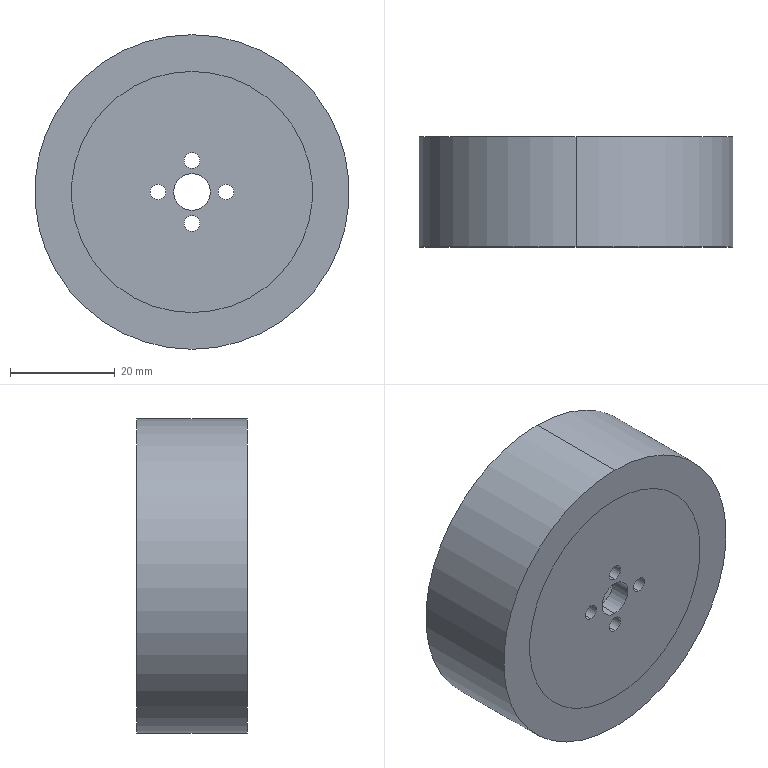Part | SolidWorks | features ICE 2, Extrusion 1 | 2 solids | 23 faces | box 60 x 21 x 60 mm | volume 35557 mm3 | cylinder 18 | plane 5 | commonest cylinder face diameters 3 x8 46 x4 7 x2 42 x2 60 x2
STEP:
#1=CARTESIAN_POINT('',(0.,21.,-21.));
#2=VERTEX_POINT('',#1);
#3=CARTESIAN_POINT('',(0.,21.,21.));
#4=VERTEX_POINT('',#3);
#5=CARTESIAN_POINT('',(0.,21.,0.));
#6=DIRECTION('',(0.,1.,0.));
#7=DIRECTION('',(0.,0.,1.));
#8=AXIS2_PLACEMENT_3D('',#5,#6,#7);
#9=CIRCLE('',#8,21.);
#10=EDGE_CURVE('',#2,#4,#9,.T.);
#11=ORIENTED_EDGE('',*,*,#10,.T.);
#12=CARTESIAN_POINT('',(0.,4.,21.));
#13=VERTEX_POINT('',#12);
#14=CARTESIAN_POINT('',(0.,21.,21.));
#15=DIRECTION('',(0.,-1.,0.));
#16=VECTOR('',#15,1000.);
#17=LINE('',#14,#16);
#18=EDGE_CURVE('',#4,#13,#17,.T.);
#19=ORIENTED_EDGE('',*,*,#18,.T.);
#20=CARTESIAN_POINT('',(0.,4.,-21.));
#21=VERTEX_POINT('',#20);
#22=CARTESIAN_POINT('',(0.,4.,0.));
#23=DIRECTION('',(0.,-1.,0.));
#24=DIRECTION('',(0.,0.,1.));
#25=AXIS2_PLACEMENT_3D('',#22,#23,#24);
#26=CIRCLE('',#25,21.);
#27=EDGE_CURVE('',#13,#21,#26,.T.);
#28=ORIENTED_EDGE('',*,*,#27,.T.);
#29=CARTESIAN_POINT('',(0.,21.,-21.));
#30=DIRECTION('',(0.,-1.,0.));
#31=VECTOR('',#30,1000.);
#32=LINE('',#29,#31);
#33=EDGE_CURVE('',#2,#21,#32,.T.);
#34=ORIENTED_EDGE('',*,*,#33,.F.);
#35=EDGE_LOOP('',(#11,#19,#28,#34));
#36=FACE_OUTER_BOUND('',#35,.T.);
#37=CARTESIAN_POINT('',(0.,21.,0.));
#38=DIRECTION('',(0.,-1.,0.));
#39=DIRECTION('',(0.,0.,-1.));
#40=AXIS2_PLACEMENT_3D('',#37,#38,#39);
#41=CYLINDRICAL_SURFACE('',#40,21.);
#42=ADVANCED_FACE('',(#36),#41,.F.);
#43=CARTESIAN_POINT('',(0.,4.,-3.5));
#44=VERTEX_POINT('',#43);
#45=CARTESIAN_POINT('',(0.,4.,3.5));
#46=VERTEX_POINT('',#45);
#47=CARTESIAN_POINT('',(0.,4.,0.));
#48=DIRECTION('',(0.,1.,0.));
#49=DIRECTION('',(0.,0.,1.));
#50=AXIS2_PLACEMENT_3D('',#47,#48,#49);
#51=CIRCLE('',#50,3.5);
#52=EDGE_CURVE('',#44,#46,#51,.T.);
#53=ORIENTED_EDGE('',*,*,#52,.T.);
#54=CARTESIAN_POINT('',(0.,0.,3.5));
#55=VERTEX_POINT('',#54);
#56=CARTESIAN_POINT('',(0.,4.,3.5));
#57=DIRECTION('',(0.,-1.,0.));
#58=VECTOR('',#57,1000.);
#59=LINE('',#56,#58);
#60=EDGE_CURVE('',#46,#55,#59,.T.);
#61=ORIENTED_EDGE('',*,*,#60,.T.);
#62=CARTESIAN_POINT('',(0.,0.,-3.5));
#63=VERTEX_POINT('',#62);
#64=CARTESIAN_POINT('',(0.,0.,0.));
#65=DIRECTION('',(0.,1.,0.));
#66=DIRECTION('',(0.,0.,1.));
#67=AXIS2_PLACEMENT_3D('',#64,#65,#66);
#68=CIRCLE('',#67,3.5);
#69=EDGE_CURVE('',#63,#55,#68,.T.);
#70=ORIENTED_EDGE('',*,*,#69,.F.);
#71=CARTESIAN_POINT('',(0.,4.,-3.5));
#72=DIRECTION('',(0.,-1.,0.));
#73=VECTOR('',#72,1000.);
#74=LINE('',#71,#73);
#75=EDGE_CURVE('',#44,#63,#74,.T.);
#76=ORIENTED_EDGE('',*,*,#75,.F.);
#77=EDGE_LOOP('',(#53,#61,#70,#76));
#78=FACE_OUTER_BOUND('',#77,.T.);
#79=CARTESIAN_POINT('',(0.,4.,0.));
#80=DIRECTION('',(0.,-1.,0.));
#81=DIRECTION('',(0.,0.,-1.));
#82=AXIS2_PLACEMENT_3D('',#79,#80,#81);
#83=CYLINDRICAL_SURFACE('',#82,3.5);
#84=ADVANCED_FACE('',(#78),#83,.F.);
#85=CARTESIAN_POINT('',(0.,4.,-7.5));
#86=VERTEX_POINT('',#85);
#87=CARTESIAN_POINT('',(0.,4.,-4.5));
#88=VERTEX_POINT('',#87);
#89=CARTESIAN_POINT('',(0.,4.,-6.));
#90=DIRECTION('',(0.,1.,0.));
#91=DIRECTION('',(0.,0.,1.));
#92=AXIS2_PLACEMENT_3D('',#89,#90,#91);
#93=CIRCLE('',#92,1.5);
#94=EDGE_CURVE('',#86,#88,#93,.T.);
#95=ORIENTED_EDGE('',*,*,#94,.T.);
#96=CARTESIAN_POINT('',(0.,0.,-4.5));
#97=VERTEX_POINT('',#96);
#98=CARTESIAN_POINT('',(0.,4.,-4.5));
#99=DIRECTION('',(0.,-1.,0.));
#100=VECTOR('',#99,1000.);
#101=LINE('',#98,#100);
#102=EDGE_CURVE('',#88,#97,#101,.T.);
#103=ORIENTED_EDGE('',*,*,#102,.T.);
#104=CARTESIAN_POINT('',(0.,0.,-7.5));
#105=VERTEX_POINT('',#104);
#106=CARTESIAN_POINT('',(0.,0.,-6.));
#107=DIRECTION('',(0.,1.,0.));
#108=DIRECTION('',(0.,0.,1.));
#109=AXIS2_PLACEMENT_3D('',#106,#107,#108);
#110=CIRCLE('',#109,1.5);
#111=EDGE_CURVE('',#105,#97,#110,.T.);
#112=ORIENTED_EDGE('',*,*,#111,.F.);
#113=CARTESIAN_POINT('',(0.,4.,-7.5));
#114=DIRECTION('',(0.,-1.,0.));
#115=VECTOR('',#114,1000.);
#116=LINE('',#113,#115);
#117=EDGE_CURVE('',#86,#105,#116,.T.);
#118=ORIENTED_EDGE('',*,*,#117,.F.);
#119=EDGE_LOOP('',(#95,#103,#112,#118));
#120=FACE_OUTER_BOUND('',#119,.T.);
#121=CARTESIAN_POINT('',(0.,4.,-6.));
#122=DIRECTION('',(0.,-1.,0.));
#123=DIRECTION('',(0.,0.,-1.));
#124=AXIS2_PLACEMENT_3D('',#121,#122,#123);
#125=CYLINDRICAL_SURFACE('',#124,1.5);
#126=ADVANCED_FACE('',(#120),#125,.F.);
#127=CARTESIAN_POINT('',(0.,4.,4.5));
#128=VERTEX_POINT('',#127);
#129=CARTESIAN_POINT('',(0.,4.,7.5));
#130=VERTEX_POINT('',#129);
#131=CARTESIAN_POINT('',(0.,4.,6.));
#132=DIRECTION('',(0.,1.,0.));
#133=DIRECTION('',(0.,0.,1.));
#134=AXIS2_PLACEMENT_3D('',#131,#132,#133);
#135=CIRCLE('',#134,1.5);
#136=EDGE_CURVE('',#128,#130,#135,.T.);
#137=ORIENTED_EDGE('',*,*,#136,.T.);
#138=CARTESIAN_POINT('',(0.,0.,7.5));
#139=VERTEX_POINT('',#138);
#140=CARTESIAN_POINT('',(0.,4.,7.5));
#141=DIRECTION('',(0.,-1.,0.));
#142=VECTOR('',#141,1000.);
#143=LINE('',#140,#142);
#144=EDGE_CURVE('',#130,#139,#143,.T.);
#145=ORIENTED_EDGE('',*,*,#144,.T.);
#146=CARTESIAN_POINT('',(0.,0.,4.5));
#147=VERTEX_POINT('',#146);
#148=CARTESIAN_POINT('',(0.,0.,6.));
#149=DIRECTION('',(0.,1.,0.));
#150=DIRECTION('',(0.,0.,1.));
#151=AXIS2_PLACEMENT_3D('',#148,#149,#150);
#152=CIRCLE('',#151,1.5);
#153=EDGE_CURVE('',#147,#139,#152,.T.);
#154=ORIENTED_EDGE('',*,*,#153,.F.);
#155=CARTESIAN_POINT('',(0.,4.,4.5));
#156=DIRECTION('',(0.,-1.,0.));
#157=VECTOR('',#156,1000.);
#158=LINE('',#155,#157);
#159=EDGE_CURVE('',#128,#147,#158,.T.);
#160=ORIENTED_EDGE('',*,*,#159,.F.);
#161=EDGE_LOOP('',(#137,#145,#154,#160));
#162=FACE_OUTER_BOUND('',#161,.T.);
#163=CARTESIAN_POINT('',(0.,4.,6.));
#164=DIRECTION('',(0.,-1.,0.));
#165=DIRECTION('',(0.,0.,-1.));
#166=AXIS2_PLACEMENT_3D('',#163,#164,#165);
#167=CYLINDRICAL_SURFACE('',#166,1.5);
#168=ADVANCED_FACE('',(#162),#167,.F.);
#169=CARTESIAN_POINT('',(-6.5,4.,-1.5));
#170=VERTEX_POINT('',#169);
#171=CARTESIAN_POINT('',(-6.5,4.,1.5));
#172=VERTEX_POINT('',#171);
#173=CARTESIAN_POINT('',(-6.5,4.,0.));
#174=DIRECTION('',(0.,1.,0.));
#175=DIRECTION('',(0.,0.,1.));
#176=AXIS2_PLACEMENT_3D('',#173,#174,#175);
#177=CIRCLE('',#176,1.5);
#178=EDGE_CURVE('',#170,#172,#177,.T.);
#179=ORIENTED_EDGE('',*,*,#178,.T.);
#180=CARTESIAN_POINT('',(-6.5,0.,1.5));
#181=VERTEX_POINT('',#180);
#182=CARTESIAN_POINT('',(-6.5,4.,1.5));
#183=DIRECTION('',(0.,-1.,0.));
#184=VECTOR('',#183,1000.);
#185=LINE('',#182,#184);
#186=EDGE_CURVE('',#172,#181,#185,.T.);
#187=ORIENTED_EDGE('',*,*,#186,.T.);
#188=CARTESIAN_POINT('',(-6.5,0.,-1.5));
#189=VERTEX_POINT('',#188);
#190=CARTESIAN_POINT('',(-6.5,0.,0.));
#191=DIRECTION('',(0.,1.,0.));
#192=DIRECTION('',(0.,0.,1.));
#193=AXIS2_PLACEMENT_3D('',#190,#191,#192);
#194=CIRCLE('',#193,1.5);
#195=EDGE_CURVE('',#189,#181,#194,.T.);
#196=ORIENTED_EDGE('',*,*,#195,.F.);
#197=CARTESIAN_POINT('',(-6.5,4.,-1.5));
#198=DIRECTION('',(0.,-1.,0.));
#199=VECTOR('',#198,1000.);
#200=LINE('',#197,#199);
#201=EDGE_CURVE('',#170,#189,#200,.T.);
#202=ORIENTED_EDGE('',*,*,#201,.F.);
#203=EDGE_LOOP('',(#179,#187,#196,#202));
#204=FACE_OUTER_BOUND('',#203,.T.);
#205=CARTESIAN_POINT('',(-6.5,4.,0.));
#206=DIRECTION('',(0.,-1.,0.));
#207=DIRECTION('',(0.,0.,-1.));
#208=AXIS2_PLACEMENT_3D('',#205,#206,#207);
#209=CYLINDRICAL_SURFACE('',#208,1.5);
#210=ADVANCED_FACE('',(#204),#209,.F.);
#211=CARTESIAN_POINT('',(6.5,4.,-1.5));
#212=VERTEX_POINT('',#211);
#213=CARTESIAN_POINT('',(6.5,4.,1.5));
#214=VERTEX_POINT('',#213);
#215=CARTESIAN_POINT('',(6.5,4.,0.));
#216=DIRECTION('',(0.,1.,0.));
#217=DIRECTION('',(0.,0.,1.));
#218=AXIS2_PLACEMENT_3D('',#215,#216,#217);
#219=CIRCLE('',#218,1.5);
#220=EDGE_CURVE('',#212,#214,#219,.T.);
#221=ORIENTED_EDGE('',*,*,#220,.T.);
#222=CARTESIAN_POINT('',(6.5,0.,1.5));
#223=VERTEX_POINT('',#222);
#224=CARTESIAN_POINT('',(6.5,4.,1.5));
#225=DIRECTION('',(0.,-1.,0.));
#226=VECTOR('',#225,1000.);
#227=LINE('',#224,#226);
#228=EDGE_CURVE('',#214,#223,#227,.T.);
#229=ORIENTED_EDGE('',*,*,#228,.T.);
#230=CARTESIAN_POINT('',(6.5,0.,-1.5));
#231=VERTEX_POINT('',#230);
#232=CARTESIAN_POINT('',(6.5,0.,0.));
#233=DIRECTION('',(0.,1.,0.));
#234=DIRECTION('',(0.,0.,1.));
#235=AXIS2_PLACEMENT_3D('',#232,#233,#234);
#236=CIRCLE('',#235,1.5);
#237=EDGE_CURVE('',#231,#223,#236,.T.);
#238=ORIENTED_EDGE('',*,*,#237,.F.);
#239=CARTESIAN_POINT('',(6.5,4.,-1.5));
#240=DIRECTION('',(0.,-1.,0.));
#241=VECTOR('',#240,1000.);
#242=LINE('',#239,#241);
#243=EDGE_CURVE('',#212,#231,#242,.T.);
#244=ORIENTED_EDGE('',*,*,#243,.F.);
#245=EDGE_LOOP('',(#221,#229,#238,#244));
#246=FACE_OUTER_BOUND('',#245,.T.);
#247=CARTESIAN_POINT('',(6.5,4.,0.));
#248=DIRECTION('',(0.,-1.,0.));
#249=DIRECTION('',(0.,0.,-1.));
#250=AXIS2_PLACEMENT_3D('',#247,#248,#249);
#251=CYLINDRICAL_SURFACE('',#250,1.5);
#252=ADVANCED_FACE('',(#246),#251,.F.);
#253=CARTESIAN_POINT('',(0.,21.,23.));
#254=VERTEX_POINT('',#253);
#255=CARTESIAN_POINT('',(0.,21.,-23.));
#256=VERTEX_POINT('',#255);
#257=CARTESIAN_POINT('',(0.,21.,0.));
#258=DIRECTION('',(0.,1.,0.));
#259=DIRECTION('',(0.,0.,1.));
#260=AXIS2_PLACEMENT_3D('',#257,#258,#259);
#261=CIRCLE('',#260,23.);
#262=EDGE_CURVE('',#254,#256,#261,.T.);
#263=ORIENTED_EDGE('',*,*,#262,.F.);
#264=CARTESIAN_POINT('',(0.,0.,23.));
#265=VERTEX_POINT('',#264);
#266=CARTESIAN_POINT('',(0.,4.,23.));
#267=DIRECTION('',(0.,-1.,0.));
#268=VECTOR('',#267,1000.);
#269=LINE('',#266,#268);
#270=EDGE_CURVE('',#254,#265,#269,.T.);
#271=ORIENTED_EDGE('',*,*,#270,.T.);
#272=CARTESIAN_POINT('',(0.,0.,-23.));
#273=VERTEX_POINT('',#272);
#274=CARTESIAN_POINT('',(0.,0.,0.));
#275=DIRECTION('',(0.,1.,0.));
#276=DIRECTION('',(0.,0.,1.));
#277=AXIS2_PLACEMENT_3D('',#274,#275,#276);
#278=CIRCLE('',#277,23.);
#279=EDGE_CURVE('',#265,#273,#278,.T.);
#280=ORIENTED_EDGE('',*,*,#279,.T.);
#281=CARTESIAN_POINT('',(0.,4.,-23.));
#282=DIRECTION('',(0.,-1.,0.));
#283=VECTOR('',#282,1000.);
#284=LINE('',#281,#283);
#285=EDGE_CURVE('',#256,#273,#284,.T.);
#286=ORIENTED_EDGE('',*,*,#285,.F.);
#287=EDGE_LOOP('',(#263,#271,#280,#286));
#288=FACE_OUTER_BOUND('',#287,.T.);
#289=CARTESIAN_POINT('',(0.,4.,0.));
#290=DIRECTION('',(0.,-1.,0.));
#291=DIRECTION('',(0.,0.,-1.));
#292=AXIS2_PLACEMENT_3D('',#289,#290,#291);
#293=CYLINDRICAL_SURFACE('',#292,23.);
#294=ADVANCED_FACE('',(#288),#293,.T.);
#295=ORIENTED_EDGE('',*,*,#52,.F.);
#296=CARTESIAN_POINT('',(0.,4.,0.));
#297=DIRECTION('',(0.,1.,0.));
#298=DIRECTION('',(0.,0.,1.));
#299=AXIS2_PLACEMENT_3D('',#296,#297,#298);
#300=CIRCLE('',#299,3.5);
#301=EDGE_CURVE('',#46,#44,#300,.T.);
#302=ORIENTED_EDGE('',*,*,#301,.F.);
#303=EDGE_LOOP('',(#295,#302));
#304=FACE_BOUND('',#303,.T.);
#305=ORIENTED_EDGE('',*,*,#136,.F.);
#306=CARTESIAN_POINT('',(0.,4.,6.));
#307=DIRECTION('',(0.,1.,0.));
#308=DIRECTION('',(0.,0.,1.));
#309=AXIS2_PLACEMENT_3D('',#306,#307,#308);
#310=CIRCLE('',#309,1.5);
#311=EDGE_CURVE('',#130,#128,#310,.T.);
#312=ORIENTED_EDGE('',*,*,#311,.F.);
#313=EDGE_LOOP('',(#305,#312));
#314=FACE_BOUND('',#313,.T.);
#315=ORIENTED_EDGE('',*,*,#220,.F.);
#316=CARTESIAN_POINT('',(6.5,4.,0.));
#317=DIRECTION('',(0.,1.,0.));
#318=DIRECTION('',(0.,0.,1.));
#319=AXIS2_PLACEMENT_3D('',#316,#317,#318);
#320=CIRCLE('',#319,1.5);
#321=EDGE_CURVE('',#214,#212,#320,.T.);
#322=ORIENTED_EDGE('',*,*,#321,.F.);
#323=EDGE_LOOP('',(#315,#322));
#324=FACE_BOUND('',#323,.T.);
#325=ORIENTED_EDGE('',*,*,#178,.F.);
#326=CARTESIAN_POINT('',(-6.5,4.,0.));
#327=DIRECTION('',(0.,1.,0.));
#328=DIRECTION('',(0.,0.,1.));
#329=AXIS2_PLACEMENT_3D('',#326,#327,#328);
#330=CIRCLE('',#329,1.5);
#331=EDGE_CURVE('',#172,#170,#330,.T.);
#332=ORIENTED_EDGE('',*,*,#331,.F.);
#333=EDGE_LOOP('',(#325,#332));
#334=FACE_BOUND('',#333,.T.);
#335=ORIENTED_EDGE('',*,*,#94,.F.);
#336=CARTESIAN_POINT('',(0.,4.,-6.));
#337=DIRECTION('',(0.,1.,0.));
#338=DIRECTION('',(0.,0.,1.));
#339=AXIS2_PLACEMENT_3D('',#336,#337,#338);
#340=CIRCLE('',#339,1.5);
#341=EDGE_CURVE('',#88,#86,#340,.T.);
#342=ORIENTED_EDGE('',*,*,#341,.F.);
#343=EDGE_LOOP('',(#335,#342));
#344=FACE_BOUND('',#343,.T.);
#345=CARTESIAN_POINT('',(0.,4.,0.));
#346=DIRECTION('',(0.,-1.,0.));
#347=DIRECTION('',(0.,0.,1.));
#348=AXIS2_PLACEMENT_3D('',#345,#346,#347);
#349=CIRCLE('',#348,21.);
#350=EDGE_CURVE('',#21,#13,#349,.T.);
#351=ORIENTED_EDGE('',*,*,#350,.F.);
#352=ORIENTED_EDGE('',*,*,#27,.F.);
#353=EDGE_LOOP('',(#351,#352));
#354=FACE_OUTER_BOUND('',#353,.T.);
#355=CARTESIAN_POINT('',(0.,4.,0.));
#356=DIRECTION('',(0.,1.,0.));
#357=DIRECTION('',(0.,0.,1.));
#358=AXIS2_PLACEMENT_3D('',#355,#356,#357);
#359=PLANE('',#358);
#360=ADVANCED_FACE('',(#304,#314,#324,#334,#344,#354),#359,.T.);
#361=CARTESIAN_POINT('',(0.,0.,0.));
#362=DIRECTION('',(0.,1.,0.));
#363=DIRECTION('',(0.,0.,1.));
#364=AXIS2_PLACEMENT_3D('',#361,#362,#363);
#365=CIRCLE('',#364,23.);
#366=EDGE_CURVE('',#273,#265,#365,.T.);
#367=ORIENTED_EDGE('',*,*,#366,.F.);
#368=ORIENTED_EDGE('',*,*,#279,.F.);
#369=EDGE_LOOP('',(#367,#368));
#370=FACE_OUTER_BOUND('',#369,.T.);
#371=ORIENTED_EDGE('',*,*,#237,.T.);
#372=CARTESIAN_POINT('',(6.5,0.,0.));
#373=DIRECTION('',(0.,1.,0.));
#374=DIRECTION('',(0.,0.,1.));
#375=AXIS2_PLACEMENT_3D('',#372,#373,#374);
#376=CIRCLE('',#375,1.5);
#377=EDGE_CURVE('',#223,#231,#376,.T.);
#378=ORIENTED_EDGE('',*,*,#377,.T.);
#379=EDGE_LOOP('',(#371,#378));
#380=FACE_BOUND('',#379,.T.);
#381=ORIENTED_EDGE('',*,*,#195,.T.);
#382=CARTESIAN_POINT('',(-6.5,0.,0.));
#383=DIRECTION('',(0.,1.,0.));
#384=DIRECTION('',(0.,0.,1.));
#385=AXIS2_PLACEMENT_3D('',#382,#383,#384);
#386=CIRCLE('',#385,1.5);
#387=EDGE_CURVE('',#181,#189,#386,.T.);
#388=ORIENTED_EDGE('',*,*,#387,.T.);
#389=EDGE_LOOP('',(#381,#388));
#390=FACE_BOUND('',#389,.T.);
#391=ORIENTED_EDGE('',*,*,#153,.T.);
#392=CARTESIAN_POINT('',(0.,0.,6.));
#393=DIRECTION('',(0.,1.,0.));
#394=DIRECTION('',(0.,0.,1.));
#395=AXIS2_PLACEMENT_3D('',#392,#393,#394);
#396=CIRCLE('',#395,1.5);
#397=EDGE_CURVE('',#139,#147,#396,.T.);
#398=ORIENTED_EDGE('',*,*,#397,.T.);
#399=EDGE_LOOP('',(#391,#398));
#400=FACE_BOUND('',#399,.T.);
#401=ORIENTED_EDGE('',*,*,#111,.T.);
#402=CARTESIAN_POINT('',(0.,0.,-6.));
#403=DIRECTION('',(0.,1.,0.));
#404=DIRECTION('',(0.,0.,1.));
#405=AXIS2_PLACEMENT_3D('',#402,#403,#404);
#406=CIRCLE('',#405,1.5);
#407=EDGE_CURVE('',#97,#105,#406,.T.);
#408=ORIENTED_EDGE('',*,*,#407,.T.);
#409=EDGE_LOOP('',(#401,#408));
#410=FACE_BOUND('',#409,.T.);
#411=ORIENTED_EDGE('',*,*,#69,.T.);
#412=CARTESIAN_POINT('',(0.,0.,0.));
#413=DIRECTION('',(0.,1.,0.));
#414=DIRECTION('',(0.,0.,1.));
#415=AXIS2_PLACEMENT_3D('',#412,#413,#414);
#416=CIRCLE('',#415,3.5);
#417=EDGE_CURVE('',#55,#63,#416,.T.);
#418=ORIENTED_EDGE('',*,*,#417,.T.);
#419=EDGE_LOOP('',(#411,#418));
#420=FACE_BOUND('',#419,.T.);
#421=CARTESIAN_POINT('',(0.,0.,0.));
#422=DIRECTION('',(0.,1.,0.));
#423=DIRECTION('',(0.,0.,1.));
#424=AXIS2_PLACEMENT_3D('',#421,#422,#423);
#425=PLANE('',#424);
#426=ADVANCED_FACE('',(#370,#380,#390,#400,#410,#420),#425,.F.);
#427=ORIENTED_EDGE('',*,*,#270,.F.);
#428=CARTESIAN_POINT('',(0.,21.,0.));
#429=DIRECTION('',(0.,1.,0.));
#430=DIRECTION('',(0.,0.,1.));
#431=AXIS2_PLACEMENT_3D('',#428,#429,#430);
#432=CIRCLE('',#431,23.);
#433=EDGE_CURVE('',#256,#254,#432,.T.);
#434=ORIENTED_EDGE('',*,*,#433,.F.);
#435=ORIENTED_EDGE('',*,*,#285,.T.);
#436=ORIENTED_EDGE('',*,*,#366,.T.);
#437=EDGE_LOOP('',(#427,#434,#435,#436));
#438=FACE_OUTER_BOUND('',#437,.T.);
#439=CARTESIAN_POINT('',(0.,4.,0.));
#440=DIRECTION('',(0.,-1.,0.));
#441=DIRECTION('',(0.,0.,-1.));
#442=AXIS2_PLACEMENT_3D('',#439,#440,#441);
#443=CYLINDRICAL_SURFACE('',#442,23.);
#444=ADVANCED_FACE('',(#438),#443,.T.);
#445=ORIENTED_EDGE('',*,*,#228,.F.);
#446=ORIENTED_EDGE('',*,*,#321,.T.);
#447=ORIENTED_EDGE('',*,*,#243,.T.);
#448=ORIENTED_EDGE('',*,*,#377,.F.);
#449=EDGE_LOOP('',(#445,#446,#447,#448));
#450=FACE_OUTER_BOUND('',#449,.T.);
#451=CARTESIAN_POINT('',(6.5,4.,0.));
#452=DIRECTION('',(0.,-1.,0.));
#453=DIRECTION('',(0.,0.,-1.));
#454=AXIS2_PLACEMENT_3D('',#451,#452,#453);
#455=CYLINDRICAL_SURFACE('',#454,1.5);
#456=ADVANCED_FACE('',(#450),#455,.F.);
#457=ORIENTED_EDGE('',*,*,#186,.F.);
#458=ORIENTED_EDGE('',*,*,#331,.T.);
#459=ORIENTED_EDGE('',*,*,#201,.T.);
#460=ORIENTED_EDGE('',*,*,#387,.F.);
#461=EDGE_LOOP('',(#457,#458,#459,#460));
#462=FACE_OUTER_BOUND('',#461,.T.);
#463=CARTESIAN_POINT('',(-6.5,4.,0.));
#464=DIRECTION('',(0.,-1.,0.));
#465=DIRECTION('',(0.,0.,-1.));
#466=AXIS2_PLACEMENT_3D('',#463,#464,#465);
#467=CYLINDRICAL_SURFACE('',#466,1.5);
#468=ADVANCED_FACE('',(#462),#467,.F.);
#469=ORIENTED_EDGE('',*,*,#144,.F.);
#470=ORIENTED_EDGE('',*,*,#311,.T.);
#471=ORIENTED_EDGE('',*,*,#159,.T.);
#472=ORIENTED_EDGE('',*,*,#397,.F.);
#473=EDGE_LOOP('',(#469,#470,#471,#472));
#474=FACE_OUTER_BOUND('',#473,.T.);
#475=CARTESIAN_POINT('',(0.,4.,6.));
#476=DIRECTION('',(0.,-1.,0.));
#477=DIRECTION('',(0.,0.,-1.));
#478=AXIS2_PLACEMENT_3D('',#475,#476,#477);
#479=CYLINDRICAL_SURFACE('',#478,1.5);
#480=ADVANCED_FACE('',(#474),#479,.F.);
#481=ORIENTED_EDGE('',*,*,#102,.F.);
#482=ORIENTED_EDGE('',*,*,#341,.T.);
#483=ORIENTED_EDGE('',*,*,#117,.T.);
#484=ORIENTED_EDGE('',*,*,#407,.F.);
#485=EDGE_LOOP('',(#481,#482,#483,#484));
#486=FACE_OUTER_BOUND('',#485,.T.);
#487=CARTESIAN_POINT('',(0.,4.,-6.));
#488=DIRECTION('',(0.,-1.,0.));
#489=DIRECTION('',(0.,0.,-1.));
#490=AXIS2_PLACEMENT_3D('',#487,#488,#489);
#491=CYLINDRICAL_SURFACE('',#490,1.5);
#492=ADVANCED_FACE('',(#486),#491,.F.);
#493=ORIENTED_EDGE('',*,*,#60,.F.);
#494=ORIENTED_EDGE('',*,*,#301,.T.);
#495=ORIENTED_EDGE('',*,*,#75,.T.);
#496=ORIENTED_EDGE('',*,*,#417,.F.);
#497=EDGE_LOOP('',(#493,#494,#495,#496));
#498=FACE_OUTER_BOUND('',#497,.T.);
#499=CARTESIAN_POINT('',(0.,4.,0.));
#500=DIRECTION('',(0.,-1.,0.));
#501=DIRECTION('',(0.,0.,-1.));
#502=AXIS2_PLACEMENT_3D('',#499,#500,#501);
#503=CYLINDRICAL_SURFACE('',#502,3.5);
#504=ADVANCED_FACE('',(#498),#503,.F.);
#505=ORIENTED_EDGE('',*,*,#433,.T.);
#506=ORIENTED_EDGE('',*,*,#262,.T.);
#507=EDGE_LOOP('',(#505,#506));
#508=FACE_OUTER_BOUND('',#507,.T.);
#509=ORIENTED_EDGE('',*,*,#10,.F.);
#510=CARTESIAN_POINT('',(0.,21.,0.));
#511=DIRECTION('',(0.,1.,0.));
#512=DIRECTION('',(0.,0.,1.));
#513=AXIS2_PLACEMENT_3D('',#510,#511,#512);
#514=CIRCLE('',#513,21.);
#515=EDGE_CURVE('',#4,#2,#514,.T.);
#516=ORIENTED_EDGE('',*,*,#515,.F.);
#517=EDGE_LOOP('',(#509,#516));
#518=FACE_BOUND('',#517,.T.);
#519=CARTESIAN_POINT('',(0.,21.,0.));
#520=DIRECTION('',(0.,1.,0.));
#521=DIRECTION('',(0.,0.,1.));
#522=AXIS2_PLACEMENT_3D('',#519,#520,#521);
#523=PLANE('',#522);
#524=ADVANCED_FACE('',(#508,#518),#523,.T.);
#525=ORIENTED_EDGE('',*,*,#18,.F.);
#526=ORIENTED_EDGE('',*,*,#515,.T.);
#527=ORIENTED_EDGE('',*,*,#33,.T.);
#528=ORIENTED_EDGE('',*,*,#350,.T.);
#529=EDGE_LOOP('',(#525,#526,#527,#528));
#530=FACE_OUTER_BOUND('',#529,.T.);
#531=CARTESIAN_POINT('',(0.,21.,0.));
#532=DIRECTION('',(0.,-1.,0.));
#533=DIRECTION('',(0.,0.,-1.));
#534=AXIS2_PLACEMENT_3D('',#531,#532,#533);
#535=CYLINDRICAL_SURFACE('',#534,21.);
#536=ADVANCED_FACE('',(#530),#535,.F.);
#537=CLOSED_SHELL('',(#42,#84,#126,#168,#210,#252,#294,#360,#426,#444,#456,#468,#480,#492,#504,#524,#536));
#538=MANIFOLD_SOLID_BREP('',#537);
#539=CARTESIAN_POINT('',(0.,21.,23.));
#540=VERTEX_POINT('',#539);
#541=CARTESIAN_POINT('',(0.,21.,-23.));
#542=VERTEX_POINT('',#541);
#543=CARTESIAN_POINT('',(0.,21.,0.));
#544=DIRECTION('',(0.,-1.,0.));
#545=DIRECTION('',(0.,0.,1.));
#546=AXIS2_PLACEMENT_3D('',#543,#544,#545);
#547=CIRCLE('',#546,23.);
#548=EDGE_CURVE('',#540,#542,#547,.T.);
#549=ORIENTED_EDGE('',*,*,#548,.F.);
#550=CARTESIAN_POINT('',(0.,0.,23.));
#551=VERTEX_POINT('',#550);
#552=CARTESIAN_POINT('',(0.,105.853,23.));
#553=DIRECTION('',(0.,-1.,0.));
#554=VECTOR('',#553,1000.);
#555=LINE('',#552,#554);
#556=EDGE_CURVE('',#540,#551,#555,.T.);
#557=ORIENTED_EDGE('',*,*,#556,.T.);
#558=CARTESIAN_POINT('',(0.,0.,-23.));
#559=VERTEX_POINT('',#558);
#560=CARTESIAN_POINT('',(0.,0.,0.));
#561=DIRECTION('',(0.,-1.,0.));
#562=DIRECTION('',(0.,0.,-1.));
#563=AXIS2_PLACEMENT_3D('',#560,#561,#562);
#564=CIRCLE('',#563,23.);
#565=EDGE_CURVE('',#551,#559,#564,.T.);
#566=ORIENTED_EDGE('',*,*,#565,.T.);
#567=CARTESIAN_POINT('',(0.,105.853,-23.));
#568=DIRECTION('',(0.,-1.,0.));
#569=VECTOR('',#568,1000.);
#570=LINE('',#567,#569);
#571=EDGE_CURVE('',#542,#559,#570,.T.);
#572=ORIENTED_EDGE('',*,*,#571,.F.);
#573=EDGE_LOOP('',(#549,#557,#566,#572));
#574=FACE_OUTER_BOUND('',#573,.T.);
#575=CARTESIAN_POINT('',(0.,105.853,0.));
#576=DIRECTION('',(0.,-1.,0.));
#577=DIRECTION('',(0.,0.,-1.));
#578=AXIS2_PLACEMENT_3D('',#575,#576,#577);
#579=CYLINDRICAL_SURFACE('',#578,23.);
#580=ADVANCED_FACE('',(#574),#579,.F.);
#581=CARTESIAN_POINT('',(0.,21.,-30.));
#582=VERTEX_POINT('',#581);
#583=CARTESIAN_POINT('',(0.,21.,30.));
#584=VERTEX_POINT('',#583);
#585=CARTESIAN_POINT('',(0.,21.,0.));
#586=DIRECTION('',(0.,-1.,0.));
#587=DIRECTION('',(0.,0.,1.));
#588=AXIS2_PLACEMENT_3D('',#585,#586,#587);
#589=CIRCLE('',#588,30.);
#590=EDGE_CURVE('',#582,#584,#589,.T.);
#591=ORIENTED_EDGE('',*,*,#590,.T.);
#592=CARTESIAN_POINT('',(0.,0.,30.));
#593=VERTEX_POINT('',#592);
#594=CARTESIAN_POINT('',(0.,105.853,30.));
#595=DIRECTION('',(0.,-1.,0.));
#596=VECTOR('',#595,1000.);
#597=LINE('',#594,#596);
#598=EDGE_CURVE('',#584,#593,#597,.T.);
#599=ORIENTED_EDGE('',*,*,#598,.T.);
#600=CARTESIAN_POINT('',(0.,0.,-30.));
#601=VERTEX_POINT('',#600);
#602=CARTESIAN_POINT('',(0.,0.,0.));
#603=DIRECTION('',(0.,-1.,0.));
#604=DIRECTION('',(0.,0.,-1.));
#605=AXIS2_PLACEMENT_3D('',#602,#603,#604);
#606=CIRCLE('',#605,30.);
#607=EDGE_CURVE('',#601,#593,#606,.T.);
#608=ORIENTED_EDGE('',*,*,#607,.F.);
#609=CARTESIAN_POINT('',(0.,105.853,-30.));
#610=DIRECTION('',(0.,-1.,0.));
#611=VECTOR('',#610,1000.);
#612=LINE('',#609,#611);
#613=EDGE_CURVE('',#582,#601,#612,.T.);
#614=ORIENTED_EDGE('',*,*,#613,.F.);
#615=EDGE_LOOP('',(#591,#599,#608,#614));
#616=FACE_OUTER_BOUND('',#615,.T.);
#617=CARTESIAN_POINT('',(0.,105.853,0.));
#618=DIRECTION('',(0.,-1.,0.));
#619=DIRECTION('',(0.,0.,-1.));
#620=AXIS2_PLACEMENT_3D('',#617,#618,#619);
#621=CYLINDRICAL_SURFACE('',#620,30.);
#622=ADVANCED_FACE('',(#616),#621,.T.);
#623=ORIENTED_EDGE('',*,*,#598,.F.);
#624=CARTESIAN_POINT('',(0.,21.,0.));
#625=DIRECTION('',(0.,-1.,0.));
#626=DIRECTION('',(0.,0.,1.));
#627=AXIS2_PLACEMENT_3D('',#624,#625,#626);
#628=CIRCLE('',#627,30.);
#629=EDGE_CURVE('',#584,#582,#628,.T.);
#630=ORIENTED_EDGE('',*,*,#629,.T.);
#631=ORIENTED_EDGE('',*,*,#613,.T.);
#632=CARTESIAN_POINT('',(0.,0.,0.));
#633=DIRECTION('',(0.,-1.,0.));
#634=DIRECTION('',(0.,0.,-1.));
#635=AXIS2_PLACEMENT_3D('',#632,#633,#634);
#636=CIRCLE('',#635,30.);
#637=EDGE_CURVE('',#593,#601,#636,.T.);
#638=ORIENTED_EDGE('',*,*,#637,.F.);
#639=EDGE_LOOP('',(#623,#630,#631,#638));
#640=FACE_OUTER_BOUND('',#639,.T.);
#641=CARTESIAN_POINT('',(0.,105.853,0.));
#642=DIRECTION('',(0.,-1.,0.));
#643=DIRECTION('',(0.,0.,-1.));
#644=AXIS2_PLACEMENT_3D('',#641,#642,#643);
#645=CYLINDRICAL_SURFACE('',#644,30.);
#646=ADVANCED_FACE('',(#640),#645,.T.);
#647=ORIENTED_EDGE('',*,*,#556,.F.);
#648=CARTESIAN_POINT('',(0.,21.,0.));
#649=DIRECTION('',(0.,-1.,0.));
#650=DIRECTION('',(0.,0.,1.));
#651=AXIS2_PLACEMENT_3D('',#648,#649,#650);
#652=CIRCLE('',#651,23.);
#653=EDGE_CURVE('',#542,#540,#652,.T.);
#654=ORIENTED_EDGE('',*,*,#653,.F.);
#655=ORIENTED_EDGE('',*,*,#571,.T.);
#656=CARTESIAN_POINT('',(0.,0.,0.));
#657=DIRECTION('',(0.,-1.,0.));
#658=DIRECTION('',(0.,0.,-1.));
#659=AXIS2_PLACEMENT_3D('',#656,#657,#658);
#660=CIRCLE('',#659,23.);
#661=EDGE_CURVE('',#559,#551,#660,.T.);
#662=ORIENTED_EDGE('',*,*,#661,.T.);
#663=EDGE_LOOP('',(#647,#654,#655,#662));
#664=FACE_OUTER_BOUND('',#663,.T.);
#665=CARTESIAN_POINT('',(0.,105.853,0.));
#666=DIRECTION('',(0.,-1.,0.));
#667=DIRECTION('',(0.,0.,-1.));
#668=AXIS2_PLACEMENT_3D('',#665,#666,#667);
#669=CYLINDRICAL_SURFACE('',#668,23.);
#670=ADVANCED_FACE('',(#664),#669,.F.);
#671=ORIENTED_EDGE('',*,*,#661,.F.);
#672=ORIENTED_EDGE('',*,*,#565,.F.);
#673=EDGE_LOOP('',(#671,#672));
#674=FACE_BOUND('',#673,.T.);
#675=ORIENTED_EDGE('',*,*,#607,.T.);
#676=ORIENTED_EDGE('',*,*,#637,.T.);
#677=EDGE_LOOP('',(#675,#676));
#678=FACE_OUTER_BOUND('',#677,.T.);
#679=CARTESIAN_POINT('',(0.,0.,0.));
#680=DIRECTION('',(0.,-1.,0.));
#681=DIRECTION('',(0.,0.,-1.));
#682=AXIS2_PLACEMENT_3D('',#679,#680,#681);
#683=PLANE('',#682);
#684=ADVANCED_FACE('',(#674,#678),#683,.T.);
#685=ORIENTED_EDGE('',*,*,#590,.F.);
#686=ORIENTED_EDGE('',*,*,#629,.F.);
#687=EDGE_LOOP('',(#685,#686));
#688=FACE_OUTER_BOUND('',#687,.T.);
#689=ORIENTED_EDGE('',*,*,#653,.T.);
#690=ORIENTED_EDGE('',*,*,#548,.T.);
#691=EDGE_LOOP('',(#689,#690));
#692=FACE_BOUND('',#691,.T.);
#693=CARTESIAN_POINT('',(0.,21.,0.));
#694=DIRECTION('',(0.,1.,0.));
#695=DIRECTION('',(0.,0.,1.));
#696=AXIS2_PLACEMENT_3D('',#693,#694,#695);
#697=PLANE('',#696);
#698=ADVANCED_FACE('',(#688,#692),#697,.T.);
#699=CLOSED_SHELL('',(#580,#622,#646,#670,#684,#698));
#700=MANIFOLD_SOLID_BREP('',#699);
#701=CARTESIAN_POINT('',(0.,0.,0.));
#702=DIRECTION('',(0.,0.,1.));
#703=DIRECTION('',(1.,0.,0.));
#704=AXIS2_PLACEMENT_3D('',#701,#702,#703);
#705=(LENGTH_UNIT()NAMED_UNIT(*)SI_UNIT(.MILLI.,.METRE.));
#706=UNCERTAINTY_MEASURE_WITH_UNIT(LENGTH_MEASURE(0.00001),#705,'','');
#707=(NAMED_UNIT(*)PLANE_ANGLE_UNIT()SI_UNIT($,.RADIAN.));
#708=(NAMED_UNIT(*)SI_UNIT($,.STERADIAN.)SOLID_ANGLE_UNIT());
#709=(GEOMETRIC_REPRESENTATION_CONTEXT(3)GLOBAL_UNCERTAINTY_ASSIGNED_CONTEXT((#706))GLOBAL_UNIT_ASSIGNED_CONTEXT((#705,#707,#708))REPRESENTATION_CONTEXT('',''));
#710=ADVANCED_BREP_SHAPE_REPRESENTATION('',(#538,#700,#704),#709);